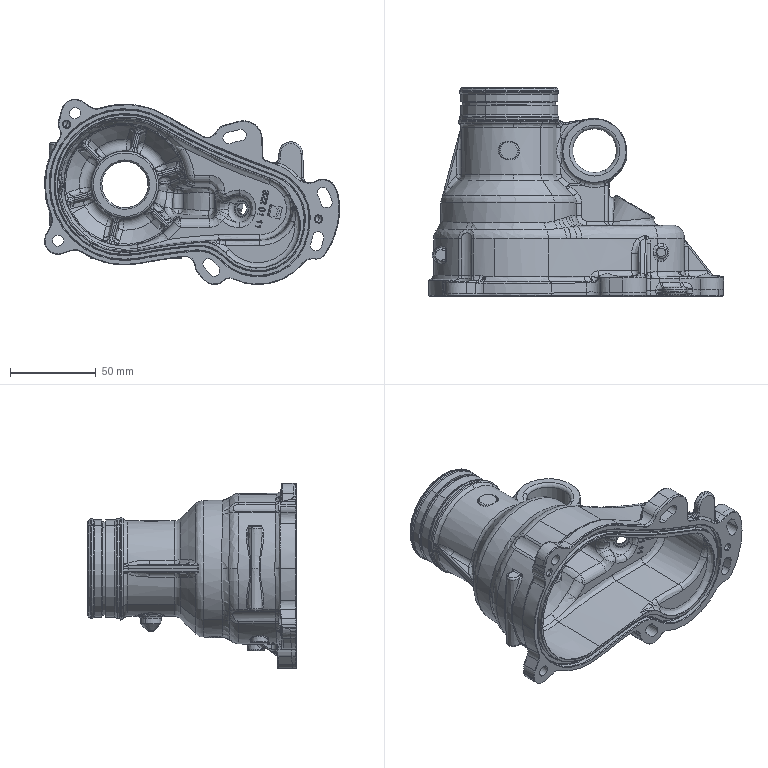Part | SolidWorks | features BaseBody 1 | 1 solid | 4449 faces | volume 242474 mm3 | plane 3071 | spline 711 | cylinder 343 | torus 144 | cone 117 | sphere 63 | commonest cylinder face diameters 6 x50 2 x49 16 x22 88 x19 8 x15 6.5 x12